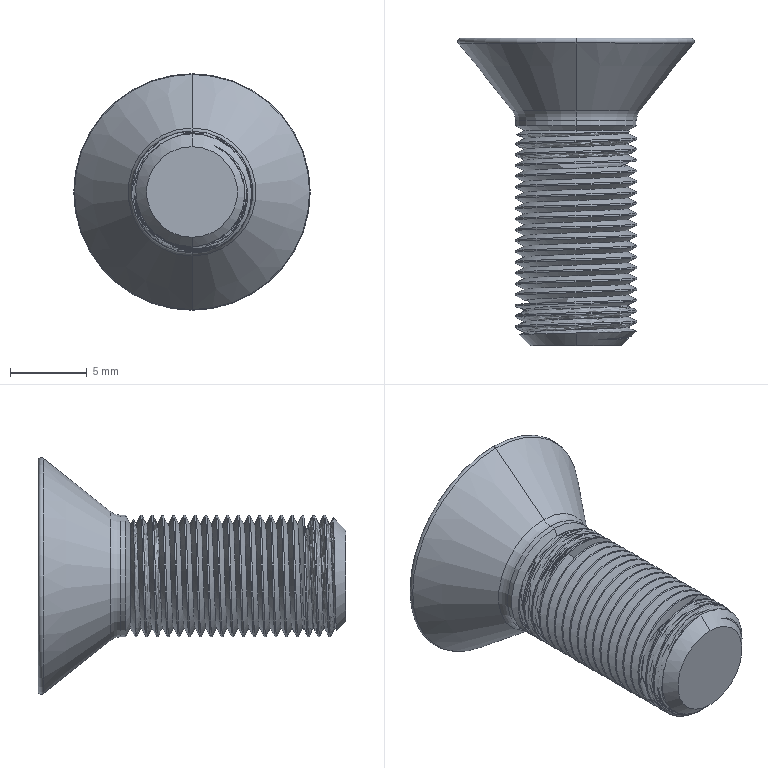Part | STEP file | Screw M8 flat head - 20mm | 1 solid | 78 faces | box 15.374 x 20 x 15.374 mm | volume 1123 mm3 | cylinder 40 | cone 15 | plane 15 | torus 4 | other 2 | spline 2 | commonest cylinder face diameters 7.9 x40